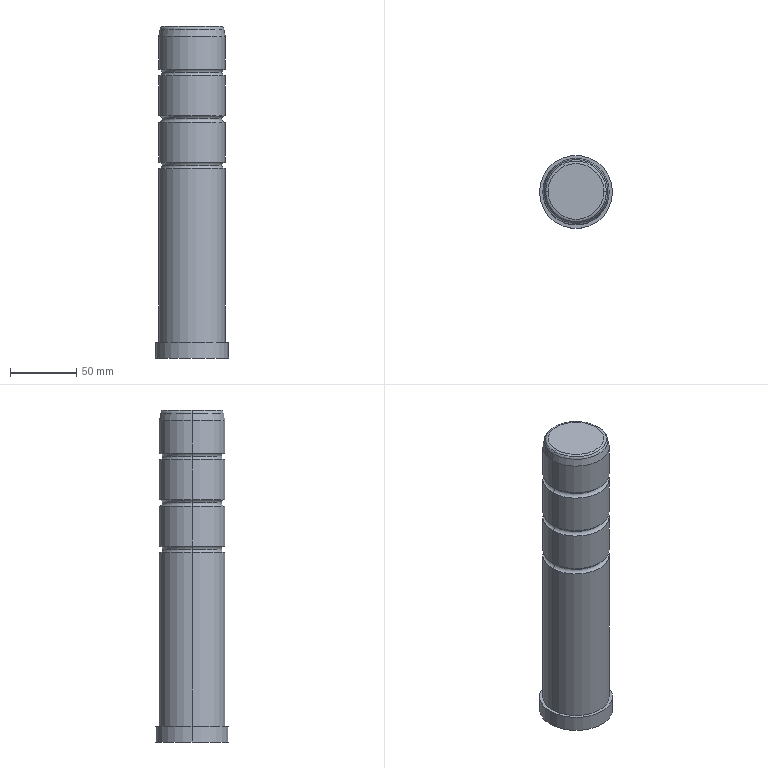Part | Creo | 1 solid | 31 faces | box 55 x 55 x 250 mm | volume 490289 mm3 | torus 16 | cylinder 10 | plane 3 | cone 2 | commonest cylinder face diameters 50 x8 55 x2
STEP:
#1=CARTESIAN_POINT('',(247.,347.,57.));
#2=VERTEX_POINT('',#1);
#3=CARTESIAN_POINT('',(297.,347.,57.));
#4=VERTEX_POINT('',#3);
#5=CARTESIAN_POINT('',(272.,347.,57.));
#6=DIRECTION('',(0.,0.,1.));
#7=DIRECTION('',(-1.,0.,0.));
#8=AXIS2_PLACEMENT_3D('',#5,#6,#7);
#9=CIRCLE('',#8,25.);
#10=EDGE_CURVE('',#2,#4,#9,.T.);
#11=ORIENTED_EDGE('',*,*,#10,.T.);
#12=CARTESIAN_POINT('',(297.,347.,27.));
#13=VERTEX_POINT('',#12);
#14=CARTESIAN_POINT('',(297.,347.,27.));
#15=DIRECTION('',(0.,0.,1.));
#16=VECTOR('',#15,30.);
#17=LINE('',#14,#16);
#18=EDGE_CURVE('',#13,#4,#17,.T.);
#19=ORIENTED_EDGE('',*,*,#18,.F.);
#20=CARTESIAN_POINT('',(247.,347.,27.));
#21=VERTEX_POINT('',#20);
#22=CARTESIAN_POINT('',(272.,347.,27.));
#23=DIRECTION('',(0.,0.,-1.));
#24=DIRECTION('',(1.,0.,0.));
#25=AXIS2_PLACEMENT_3D('',#22,#23,#24);
#26=CIRCLE('',#25,25.);
#27=EDGE_CURVE('',#13,#21,#26,.T.);
#28=ORIENTED_EDGE('',*,*,#27,.T.);
#29=CARTESIAN_POINT('',(247.,347.,27.));
#30=DIRECTION('',(0.,0.,1.));
#31=VECTOR('',#30,30.);
#32=LINE('',#29,#31);
#33=EDGE_CURVE('',#21,#2,#32,.T.);
#34=ORIENTED_EDGE('',*,*,#33,.T.);
#35=EDGE_LOOP('',(#11,#19,#28,#34));
#36=FACE_OUTER_BOUND('',#35,.F.);
#37=CARTESIAN_POINT('',(272.,347.,-108.5));
#38=DIRECTION('',(0.,0.,1.));
#39=DIRECTION('',(-1.,0.,0.));
#40=AXIS2_PLACEMENT_3D('',#37,#38,#39);
#41=CYLINDRICAL_SURFACE('',#40,25.);
#42=ADVANCED_FACE('',(#36),#41,.T.);
#43=ORIENTED_EDGE('',*,*,#10,.F.);
#44=CARTESIAN_POINT('',(249.5,347.,59.5));
#45=VERTEX_POINT('',#44);
#46=CARTESIAN_POINT('',(247.,347.,59.5));
#47=DIRECTION('',(0.,1.,0.));
#48=DIRECTION('',(1.,0.,0.));
#49=AXIS2_PLACEMENT_3D('',#46,#47,#48);
#50=CIRCLE('',#49,2.5);
#51=EDGE_CURVE('',#45,#2,#50,.T.);
#52=ORIENTED_EDGE('',*,*,#51,.F.);
#53=CARTESIAN_POINT('',(294.5,347.,59.5));
#54=VERTEX_POINT('',#53);
#55=CARTESIAN_POINT('',(272.,347.,59.5));
#56=DIRECTION('',(0.,0.,1.));
#57=DIRECTION('',(-1.,0.,0.));
#58=AXIS2_PLACEMENT_3D('',#55,#56,#57);
#59=CIRCLE('',#58,22.5);
#60=EDGE_CURVE('',#45,#54,#59,.T.);
#61=ORIENTED_EDGE('',*,*,#60,.T.);
#62=CARTESIAN_POINT('',(297.,347.,59.5));
#63=DIRECTION('',(0.,-1.,0.));
#64=DIRECTION('',(-1.,0.,0.));
#65=AXIS2_PLACEMENT_3D('',#62,#63,#64);
#66=CIRCLE('',#65,2.5);
#67=EDGE_CURVE('',#54,#4,#66,.T.);
#68=ORIENTED_EDGE('',*,*,#67,.T.);
#69=EDGE_LOOP('',(#43,#52,#61,#68));
#70=FACE_OUTER_BOUND('',#69,.F.);
#71=CARTESIAN_POINT('',(272.,347.,59.5));
#72=DIRECTION('',(0.,0.,1.));
#73=DIRECTION('',(-1.,0.,0.));
#74=AXIS2_PLACEMENT_3D('',#71,#72,#73);
#75=TOROIDAL_SURFACE('',#74,25.,2.5);
#76=ADVANCED_FACE('',(#70),#75,.F.);
#77=CARTESIAN_POINT('',(272.,347.,57.));
#78=DIRECTION('',(0.,0.,1.));
#79=DIRECTION('',(1.,0.,0.));
#80=AXIS2_PLACEMENT_3D('',#77,#78,#79);
#81=CIRCLE('',#80,25.);
#82=EDGE_CURVE('',#4,#2,#81,.T.);
#83=ORIENTED_EDGE('',*,*,#82,.F.);
#84=ORIENTED_EDGE('',*,*,#67,.F.);
#85=CARTESIAN_POINT('',(272.,347.,59.5));
#86=DIRECTION('',(0.,0.,1.));
#87=DIRECTION('',(1.,0.,0.));
#88=AXIS2_PLACEMENT_3D('',#85,#86,#87);
#89=CIRCLE('',#88,22.5);
#90=EDGE_CURVE('',#54,#45,#89,.T.);
#91=ORIENTED_EDGE('',*,*,#90,.T.);
#92=ORIENTED_EDGE('',*,*,#51,.T.);
#93=EDGE_LOOP('',(#83,#84,#91,#92));
#94=FACE_OUTER_BOUND('',#93,.F.);
#95=CARTESIAN_POINT('',(272.,347.,59.5));
#96=DIRECTION('',(0.,0.,1.));
#97=DIRECTION('',(-1.,0.,0.));
#98=AXIS2_PLACEMENT_3D('',#95,#96,#97);
#99=TOROIDAL_SURFACE('',#98,25.,2.5);
#100=ADVANCED_FACE('',(#94),#99,.F.);
#101=ORIENTED_EDGE('',*,*,#82,.T.);
#102=ORIENTED_EDGE('',*,*,#33,.F.);
#103=CARTESIAN_POINT('',(272.,347.,27.));
#104=DIRECTION('',(0.,0.,-1.));
#105=DIRECTION('',(-1.,0.,0.));
#106=AXIS2_PLACEMENT_3D('',#103,#104,#105);
#107=CIRCLE('',#106,25.);
#108=EDGE_CURVE('',#21,#13,#107,.T.);
#109=ORIENTED_EDGE('',*,*,#108,.T.);
#110=ORIENTED_EDGE('',*,*,#18,.T.);
#111=EDGE_LOOP('',(#101,#102,#109,#110));
#112=FACE_OUTER_BOUND('',#111,.F.);
#113=CARTESIAN_POINT('',(272.,347.,-108.5));
#114=DIRECTION('',(0.,0.,1.));
#115=DIRECTION('',(-1.,0.,0.));
#116=AXIS2_PLACEMENT_3D('',#113,#114,#115);
#117=CYLINDRICAL_SURFACE('',#116,25.);
#118=ADVANCED_FACE('',(#112),#117,.T.);
#119=ORIENTED_EDGE('',*,*,#108,.F.);
#120=CARTESIAN_POINT('',(249.5,347.,24.5));
#121=VERTEX_POINT('',#120);
#122=CARTESIAN_POINT('',(247.,347.,24.5));
#123=DIRECTION('',(0.,1.,0.));
#124=DIRECTION('',(0.,0.,1.));
#125=AXIS2_PLACEMENT_3D('',#122,#123,#124);
#126=CIRCLE('',#125,2.5);
#127=EDGE_CURVE('',#21,#121,#126,.T.);
#128=ORIENTED_EDGE('',*,*,#127,.T.);
#129=CARTESIAN_POINT('',(294.5,347.,24.5));
#130=VERTEX_POINT('',#129);
#131=CARTESIAN_POINT('',(272.,347.,24.5));
#132=DIRECTION('',(0.,0.,1.));
#133=DIRECTION('',(1.,0.,0.));
#134=AXIS2_PLACEMENT_3D('',#131,#132,#133);
#135=CIRCLE('',#134,22.5);
#136=EDGE_CURVE('',#130,#121,#135,.T.);
#137=ORIENTED_EDGE('',*,*,#136,.F.);
#138=CARTESIAN_POINT('',(297.,347.,24.5));
#139=DIRECTION('',(0.,-1.,0.));
#140=DIRECTION('',(0.,0.,1.));
#141=AXIS2_PLACEMENT_3D('',#138,#139,#140);
#142=CIRCLE('',#141,2.5);
#143=EDGE_CURVE('',#13,#130,#142,.T.);
#144=ORIENTED_EDGE('',*,*,#143,.F.);
#145=EDGE_LOOP('',(#119,#128,#137,#144));
#146=FACE_OUTER_BOUND('',#145,.F.);
#147=CARTESIAN_POINT('',(272.,347.,24.5));
#148=DIRECTION('',(0.,0.,1.));
#149=DIRECTION('',(-1.,0.,0.));
#150=AXIS2_PLACEMENT_3D('',#147,#148,#149);
#151=TOROIDAL_SURFACE('',#150,25.,2.5);
#152=ADVANCED_FACE('',(#146),#151,.F.);
#153=ORIENTED_EDGE('',*,*,#27,.F.);
#154=ORIENTED_EDGE('',*,*,#143,.T.);
#155=CARTESIAN_POINT('',(272.,347.,24.5));
#156=DIRECTION('',(0.,0.,1.));
#157=DIRECTION('',(-1.,0.,0.));
#158=AXIS2_PLACEMENT_3D('',#155,#156,#157);
#159=CIRCLE('',#158,22.5);
#160=EDGE_CURVE('',#121,#130,#159,.T.);
#161=ORIENTED_EDGE('',*,*,#160,.F.);
#162=ORIENTED_EDGE('',*,*,#127,.F.);
#163=EDGE_LOOP('',(#153,#154,#161,#162));
#164=FACE_OUTER_BOUND('',#163,.F.);
#165=CARTESIAN_POINT('',(272.,347.,24.5));
#166=DIRECTION('',(0.,0.,1.));
#167=DIRECTION('',(-1.,0.,0.));
#168=AXIS2_PLACEMENT_3D('',#165,#166,#167);
#169=TOROIDAL_SURFACE('',#168,25.,2.5);
#170=ADVANCED_FACE('',(#164),#169,.F.);
#171=CARTESIAN_POINT('',(247.,347.,22.));
#172=VERTEX_POINT('',#171);
#173=CARTESIAN_POINT('',(297.,347.,22.));
#174=VERTEX_POINT('',#173);
#175=CARTESIAN_POINT('',(272.,347.,22.));
#176=DIRECTION('',(0.,0.,1.));
#177=DIRECTION('',(-1.,0.,0.));
#178=AXIS2_PLACEMENT_3D('',#175,#176,#177);
#179=CIRCLE('',#178,25.);
#180=EDGE_CURVE('',#172,#174,#179,.T.);
#181=ORIENTED_EDGE('',*,*,#180,.F.);
#182=CARTESIAN_POINT('',(247.,347.,24.5));
#183=DIRECTION('',(0.,1.,0.));
#184=DIRECTION('',(1.,0.,0.));
#185=AXIS2_PLACEMENT_3D('',#182,#183,#184);
#186=CIRCLE('',#185,2.5);
#187=EDGE_CURVE('',#121,#172,#186,.T.);
#188=ORIENTED_EDGE('',*,*,#187,.F.);
#189=ORIENTED_EDGE('',*,*,#160,.T.);
#190=CARTESIAN_POINT('',(297.,347.,24.5));
#191=DIRECTION('',(0.,-1.,0.));
#192=DIRECTION('',(-1.,0.,0.));
#193=AXIS2_PLACEMENT_3D('',#190,#191,#192);
#194=CIRCLE('',#193,2.5);
#195=EDGE_CURVE('',#130,#174,#194,.T.);
#196=ORIENTED_EDGE('',*,*,#195,.T.);
#197=EDGE_LOOP('',(#181,#188,#189,#196));
#198=FACE_OUTER_BOUND('',#197,.F.);
#199=CARTESIAN_POINT('',(272.,347.,24.5));
#200=DIRECTION('',(0.,0.,1.));
#201=DIRECTION('',(-1.,0.,0.));
#202=AXIS2_PLACEMENT_3D('',#199,#200,#201);
#203=TOROIDAL_SURFACE('',#202,25.,2.5);
#204=ADVANCED_FACE('',(#198),#203,.F.);
#205=CARTESIAN_POINT('',(297.,347.,-108.5));
#206=VERTEX_POINT('',#205);
#207=CARTESIAN_POINT('',(247.,347.,-108.5));
#208=VERTEX_POINT('',#207);
#209=CARTESIAN_POINT('',(272.,347.,-108.5));
#210=DIRECTION('',(0.,0.,-1.));
#211=DIRECTION('',(1.,0.,0.));
#212=AXIS2_PLACEMENT_3D('',#209,#210,#211);
#213=CIRCLE('',#212,25.);
#214=EDGE_CURVE('',#206,#208,#213,.T.);
#215=ORIENTED_EDGE('',*,*,#214,.T.);
#216=CARTESIAN_POINT('',(247.,347.,-108.5));
#217=DIRECTION('',(0.,0.,1.));
#218=VECTOR('',#217,130.5);
#219=LINE('',#216,#218);
#220=EDGE_CURVE('',#208,#172,#219,.T.);
#221=ORIENTED_EDGE('',*,*,#220,.T.);
#222=ORIENTED_EDGE('',*,*,#180,.T.);
#223=CARTESIAN_POINT('',(297.,347.,-108.5));
#224=DIRECTION('',(0.,0.,1.));
#225=VECTOR('',#224,130.5);
#226=LINE('',#223,#225);
#227=EDGE_CURVE('',#206,#174,#226,.T.);
#228=ORIENTED_EDGE('',*,*,#227,.F.);
#229=EDGE_LOOP('',(#215,#221,#222,#228));
#230=FACE_OUTER_BOUND('',#229,.F.);
#231=CARTESIAN_POINT('',(272.,347.,-108.5));
#232=DIRECTION('',(0.,0.,1.));
#233=DIRECTION('',(-1.,0.,0.));
#234=AXIS2_PLACEMENT_3D('',#231,#232,#233);
#235=CYLINDRICAL_SURFACE('',#234,25.);
#236=ADVANCED_FACE('',(#230),#235,.T.);
#237=CARTESIAN_POINT('',(299.5,347.,-108.5));
#238=VERTEX_POINT('',#237);
#239=CARTESIAN_POINT('',(244.5,347.,-108.5));
#240=VERTEX_POINT('',#239);
#241=CARTESIAN_POINT('',(272.,347.,-108.5));
#242=DIRECTION('',(0.,0.,1.));
#243=DIRECTION('',(1.,0.,0.));
#244=AXIS2_PLACEMENT_3D('',#241,#242,#243);
#245=CIRCLE('',#244,27.5);
#246=EDGE_CURVE('',#238,#240,#245,.T.);
#247=ORIENTED_EDGE('',*,*,#246,.F.);
#248=CARTESIAN_POINT('',(272.,347.,-108.5));
#249=DIRECTION('',(0.,0.,1.));
#250=DIRECTION('',(-1.,0.,0.));
#251=AXIS2_PLACEMENT_3D('',#248,#249,#250);
#252=CIRCLE('',#251,27.5);
#253=EDGE_CURVE('',#240,#238,#252,.T.);
#254=ORIENTED_EDGE('',*,*,#253,.F.);
#255=EDGE_LOOP('',(#247,#254));
#256=FACE_OUTER_BOUND('',#255,.F.);
#257=CARTESIAN_POINT('',(272.,347.,-108.5));
#258=DIRECTION('',(0.,0.,-1.));
#259=DIRECTION('',(-1.,0.,0.));
#260=AXIS2_PLACEMENT_3D('',#257,#258,#259);
#261=CIRCLE('',#260,25.);
#262=EDGE_CURVE('',#208,#206,#261,.T.);
#263=ORIENTED_EDGE('',*,*,#262,.F.);
#264=ORIENTED_EDGE('',*,*,#214,.F.);
#265=EDGE_LOOP('',(#263,#264));
#266=FACE_BOUND('',#265,.F.);
#267=CARTESIAN_POINT('',(272.,347.,-108.5));
#268=DIRECTION('',(0.,0.,-1.));
#269=DIRECTION('',(1.,0.,0.));
#270=AXIS2_PLACEMENT_3D('',#267,#268,#269);
#271=PLANE('',#270);
#272=ADVANCED_FACE('',(#256,#266),#271,.F.);
#273=ORIENTED_EDGE('',*,*,#262,.T.);
#274=ORIENTED_EDGE('',*,*,#227,.T.);
#275=CARTESIAN_POINT('',(272.,347.,22.));
#276=DIRECTION('',(0.,0.,1.));
#277=DIRECTION('',(1.,0.,0.));
#278=AXIS2_PLACEMENT_3D('',#275,#276,#277);
#279=CIRCLE('',#278,25.);
#280=EDGE_CURVE('',#174,#172,#279,.T.);
#281=ORIENTED_EDGE('',*,*,#280,.T.);
#282=ORIENTED_EDGE('',*,*,#220,.F.);
#283=EDGE_LOOP('',(#273,#274,#281,#282));
#284=FACE_OUTER_BOUND('',#283,.F.);
#285=CARTESIAN_POINT('',(272.,347.,-108.5));
#286=DIRECTION('',(0.,0.,1.));
#287=DIRECTION('',(-1.,0.,0.));
#288=AXIS2_PLACEMENT_3D('',#285,#286,#287);
#289=CYLINDRICAL_SURFACE('',#288,25.);
#290=ADVANCED_FACE('',(#284),#289,.T.);
#291=ORIENTED_EDGE('',*,*,#280,.F.);
#292=ORIENTED_EDGE('',*,*,#195,.F.);
#293=ORIENTED_EDGE('',*,*,#136,.T.);
#294=ORIENTED_EDGE('',*,*,#187,.T.);
#295=EDGE_LOOP('',(#291,#292,#293,#294));
#296=FACE_OUTER_BOUND('',#295,.F.);
#297=CARTESIAN_POINT('',(272.,347.,24.5));
#298=DIRECTION('',(0.,0.,1.));
#299=DIRECTION('',(-1.,0.,0.));
#300=AXIS2_PLACEMENT_3D('',#297,#298,#299);
#301=TOROIDAL_SURFACE('',#300,25.,2.5);
#302=ADVANCED_FACE('',(#296),#301,.F.);
#303=ORIENTED_EDGE('',*,*,#246,.T.);
#304=CARTESIAN_POINT('',(244.5,347.,-120.5));
#305=VERTEX_POINT('',#304);
#306=CARTESIAN_POINT('',(244.5,347.,-108.5));
#307=DIRECTION('',(0.,0.,-1.));
#308=VECTOR('',#307,12.);
#309=LINE('',#306,#308);
#310=EDGE_CURVE('',#240,#305,#309,.T.);
#311=ORIENTED_EDGE('',*,*,#310,.T.);
#312=CARTESIAN_POINT('',(299.5,347.,-120.5));
#313=VERTEX_POINT('',#312);
#314=CARTESIAN_POINT('',(272.,347.,-120.5));
#315=DIRECTION('',(0.,0.,-1.));
#316=DIRECTION('',(-1.,0.,0.));
#317=AXIS2_PLACEMENT_3D('',#314,#315,#316);
#318=CIRCLE('',#317,27.5);
#319=EDGE_CURVE('',#305,#313,#318,.T.);
#320=ORIENTED_EDGE('',*,*,#319,.T.);
#321=CARTESIAN_POINT('',(299.5,347.,-108.5));
#322=DIRECTION('',(0.,0.,-1.));
#323=VECTOR('',#322,12.);
#324=LINE('',#321,#323);
#325=EDGE_CURVE('',#238,#313,#324,.T.);
#326=ORIENTED_EDGE('',*,*,#325,.F.);
#327=EDGE_LOOP('',(#303,#311,#320,#326));
#328=FACE_OUTER_BOUND('',#327,.F.);
#329=CARTESIAN_POINT('',(272.,347.,-108.5));
#330=DIRECTION('',(0.,0.,-1.));
#331=DIRECTION('',(1.,0.,0.));
#332=AXIS2_PLACEMENT_3D('',#329,#330,#331);
#333=CYLINDRICAL_SURFACE('',#332,27.5);
#334=ADVANCED_FACE('',(#328),#333,.T.);
#335=ORIENTED_EDGE('',*,*,#253,.T.);
#336=ORIENTED_EDGE('',*,*,#325,.T.);
#337=CARTESIAN_POINT('',(272.,347.,-120.5));
#338=DIRECTION('',(0.,0.,-1.));
#339=DIRECTION('',(1.,0.,0.));
#340=AXIS2_PLACEMENT_3D('',#337,#338,#339);
#341=CIRCLE('',#340,27.5);
#342=EDGE_CURVE('',#313,#305,#341,.T.);
#343=ORIENTED_EDGE('',*,*,#342,.T.);
#344=ORIENTED_EDGE('',*,*,#310,.F.);
#345=EDGE_LOOP('',(#335,#336,#343,#344));
#346=FACE_OUTER_BOUND('',#345,.F.);
#347=CARTESIAN_POINT('',(272.,347.,-108.5));
#348=DIRECTION('',(0.,0.,-1.));
#349=DIRECTION('',(1.,0.,0.));
#350=AXIS2_PLACEMENT_3D('',#347,#348,#349);
#351=CYLINDRICAL_SURFACE('',#350,27.5);
#352=ADVANCED_FACE('',(#346),#351,.T.);
#353=ORIENTED_EDGE('',*,*,#342,.F.);
#354=ORIENTED_EDGE('',*,*,#319,.F.);
#355=EDGE_LOOP('',(#353,#354));
#356=FACE_OUTER_BOUND('',#355,.F.);
#357=CARTESIAN_POINT('',(272.,347.,-120.5));
#358=DIRECTION('',(0.,0.,-1.));
#359=DIRECTION('',(1.,0.,0.));
#360=AXIS2_PLACEMENT_3D('',#357,#358,#359);
#361=PLANE('',#360);
#362=ADVANCED_FACE('',(#356),#361,.T.);
#363=CARTESIAN_POINT('',(247.,347.,62.));
#364=VERTEX_POINT('',#363);
#365=CARTESIAN_POINT('',(297.,347.,62.));
#366=VERTEX_POINT('',#365);
#367=CARTESIAN_POINT('',(272.,347.,62.));
#368=DIRECTION('',(0.,0.,-1.));
#369=DIRECTION('',(-1.,0.,0.));
#370=AXIS2_PLACEMENT_3D('',#367,#368,#369);
#371=CIRCLE('',#370,25.);
#372=EDGE_CURVE('',#364,#366,#371,.T.);
#373=ORIENTED_EDGE('',*,*,#372,.F.);
#374=CARTESIAN_POINT('',(247.,347.,59.5));
#375=DIRECTION('',(0.,1.,0.));
#376=DIRECTION('',(0.,0.,1.));
#377=AXIS2_PLACEMENT_3D('',#374,#375,#376);
#378=CIRCLE('',#377,2.5);
#379=EDGE_CURVE('',#364,#45,#378,.T.);
#380=ORIENTED_EDGE('',*,*,#379,.T.);
#381=ORIENTED_EDGE('',*,*,#90,.F.);
#382=CARTESIAN_POINT('',(297.,347.,59.5));
#383=DIRECTION('',(0.,-1.,0.));
#384=DIRECTION('',(0.,0.,1.));
#385=AXIS2_PLACEMENT_3D('',#382,#383,#384);
#386=CIRCLE('',#385,2.5);
#387=EDGE_CURVE('',#366,#54,#386,.T.);
#388=ORIENTED_EDGE('',*,*,#387,.F.);
#389=EDGE_LOOP('',(#373,#380,#381,#388));
#390=FACE_OUTER_BOUND('',#389,.F.);
#391=CARTESIAN_POINT('',(272.,347.,59.5));
#392=DIRECTION('',(0.,0.,1.));
#393=DIRECTION('',(-1.,0.,0.));
#394=AXIS2_PLACEMENT_3D('',#391,#392,#393);
#395=TOROIDAL_SURFACE('',#394,25.,2.5);
#396=ADVANCED_FACE('',(#390),#395,.F.);
#397=CARTESIAN_POINT('',(297.,347.,92.));
#398=VERTEX_POINT('',#397);
#399=CARTESIAN_POINT('',(247.,347.,92.));
#400=VERTEX_POINT('',#399);
#401=CARTESIAN_POINT('',(272.,347.,92.));
#402=DIRECTION('',(0.,0.,1.));
#403=DIRECTION('',(1.,0.,0.));
#404=AXIS2_PLACEMENT_3D('',#401,#402,#403);
#405=CIRCLE('',#404,25.);
#406=EDGE_CURVE('',#398,#400,#405,.T.);
#407=ORIENTED_EDGE('',*,*,#406,.T.);
#408=CARTESIAN_POINT('',(247.,347.,62.));
#409=DIRECTION('',(0.,0.,1.));
#410=VECTOR('',#409,30.);
#411=LINE('',#408,#410);
#412=EDGE_CURVE('',#364,#400,#411,.T.);
#413=ORIENTED_EDGE('',*,*,#412,.F.);
#414=ORIENTED_EDGE('',*,*,#372,.T.);
#415=CARTESIAN_POINT('',(297.,347.,62.));
#416=DIRECTION('',(0.,0.,1.));
#417=VECTOR('',#416,30.);
#418=LINE('',#415,#417);
#419=EDGE_CURVE('',#366,#398,#418,.T.);
#420=ORIENTED_EDGE('',*,*,#419,.T.);
#421=EDGE_LOOP('',(#407,#413,#414,#420));
#422=FACE_OUTER_BOUND('',#421,.F.);
#423=CARTESIAN_POINT('',(272.,347.,-108.5));
#424=DIRECTION('',(0.,0.,1.));
#425=DIRECTION('',(-1.,0.,0.));
#426=AXIS2_PLACEMENT_3D('',#423,#424,#425);
#427=CYLINDRICAL_SURFACE('',#426,25.);
#428=ADVANCED_FACE('',(#422),#427,.T.);
#429=ORIENTED_EDGE('',*,*,#406,.F.);
#430=CARTESIAN_POINT('',(294.5,347.,94.5));
#431=VERTEX_POINT('',#430);
#432=CARTESIAN_POINT('',(297.,347.,94.5));
#433=DIRECTION('',(0.,-1.,0.));
#434=DIRECTION('',(-1.,0.,0.));
#435=AXIS2_PLACEMENT_3D('',#432,#433,#434);
#436=CIRCLE('',#435,2.5);
#437=EDGE_CURVE('',#431,#398,#436,.T.);
#438=ORIENTED_EDGE('',*,*,#437,.F.);
#439=CARTESIAN_POINT('',(249.5,347.,94.5));
#440=VERTEX_POINT('',#439);
#441=CARTESIAN_POINT('',(272.,347.,94.5));
#442=DIRECTION('',(0.,0.,1.));
#443=DIRECTION('',(1.,0.,0.));
#444=AXIS2_PLACEMENT_3D('',#441,#442,#443);
#445=CIRCLE('',#444,22.5);
#446=EDGE_CURVE('',#431,#440,#445,.T.);
#447=ORIENTED_EDGE('',*,*,#446,.T.);
#448=CARTESIAN_POINT('',(247.,347.,94.5));
#449=DIRECTION('',(0.,1.,0.));
#450=DIRECTION('',(1.,0.,0.));
#451=AXIS2_PLACEMENT_3D('',#448,#449,#450);
#452=CIRCLE('',#451,2.5);
#453=EDGE_CURVE('',#440,#400,#452,.T.);
#454=ORIENTED_EDGE('',*,*,#453,.T.);
#455=EDGE_LOOP('',(#429,#438,#447,#454));
#456=FACE_OUTER_BOUND('',#455,.F.);
#457=CARTESIAN_POINT('',(272.,347.,94.5));
#458=DIRECTION('',(0.,0.,1.));
#459=DIRECTION('',(-1.,0.,0.));
#460=AXIS2_PLACEMENT_3D('',#457,#458,#459);
#461=TOROIDAL_SURFACE('',#460,25.,2.5);
#462=ADVANCED_FACE('',(#456),#461,.F.);
#463=CARTESIAN_POINT('',(272.,347.,92.));
#464=DIRECTION('',(0.,0.,1.));
#465=DIRECTION('',(-1.,0.,0.));
#466=AXIS2_PLACEMENT_3D('',#463,#464,#465);
#467=CIRCLE('',#466,25.);
#468=EDGE_CURVE('',#400,#398,#467,.T.);
#469=ORIENTED_EDGE('',*,*,#468,.F.);
#470=ORIENTED_EDGE('',*,*,#453,.F.);
#471=CARTESIAN_POINT('',(272.,347.,94.5));
#472=DIRECTION('',(0.,0.,1.));
#473=DIRECTION('',(-1.,0.,0.));
#474=AXIS2_PLACEMENT_3D('',#471,#472,#473);
#475=CIRCLE('',#474,22.5);
#476=EDGE_CURVE('',#440,#431,#475,.T.);
#477=ORIENTED_EDGE('',*,*,#476,.T.);
#478=ORIENTED_EDGE('',*,*,#437,.T.);
#479=EDGE_LOOP('',(#469,#470,#477,#478));
#480=FACE_OUTER_BOUND('',#479,.F.);
#481=CARTESIAN_POINT('',(272.,347.,94.5));
#482=DIRECTION('',(0.,0.,1.));
#483=DIRECTION('',(-1.,0.,0.));
#484=AXIS2_PLACEMENT_3D('',#481,#482,#483);
#485=TOROIDAL_SURFACE('',#484,25.,2.5);
#486=ADVANCED_FACE('',(#480),#485,.F.);
#487=ORIENTED_EDGE('',*,*,#468,.T.);
#488=ORIENTED_EDGE('',*,*,#419,.F.);
#489=CARTESIAN_POINT('',(272.,347.,62.));
#490=DIRECTION('',(0.,0.,-1.));
#491=DIRECTION('',(1.,0.,0.));
#492=AXIS2_PLACEMENT_3D('',#489,#490,#491);
#493=CIRCLE('',#492,25.);
#494=EDGE_CURVE('',#366,#364,#493,.T.);
#495=ORIENTED_EDGE('',*,*,#494,.T.);
#496=ORIENTED_EDGE('',*,*,#412,.T.);
#497=EDGE_LOOP('',(#487,#488,#495,#496));
#498=FACE_OUTER_BOUND('',#497,.F.);
#499=CARTESIAN_POINT('',(272.,347.,-108.5));
#500=DIRECTION('',(0.,0.,1.));
#501=DIRECTION('',(-1.,0.,0.));
#502=AXIS2_PLACEMENT_3D('',#499,#500,#501);
#503=CYLINDRICAL_SURFACE('',#502,25.);
#504=ADVANCED_FACE('',(#498),#503,.T.);
#505=ORIENTED_EDGE('',*,*,#494,.F.);
#506=ORIENTED_EDGE('',*,*,#387,.T.);
#507=ORIENTED_EDGE('',*,*,#60,.F.);
#508=ORIENTED_EDGE('',*,*,#379,.F.);
#509=EDGE_LOOP('',(#505,#506,#507,#508));
#510=FACE_OUTER_BOUND('',#509,.F.);
#511=CARTESIAN_POINT('',(272.,347.,59.5));
#512=DIRECTION('',(0.,0.,1.));
#513=DIRECTION('',(-1.,0.,0.));
#514=AXIS2_PLACEMENT_3D('',#511,#512,#513);
#515=TOROIDAL_SURFACE('',#514,25.,2.5);
#516=ADVANCED_FACE('',(#510),#515,.F.);
#517=CARTESIAN_POINT('',(297.,347.,97.));
#518=VERTEX_POINT('',#517);
#519=CARTESIAN_POINT('',(247.,347.,97.));
#520=VERTEX_POINT('',#519);
#521=CARTESIAN_POINT('',(272.,347.,97.));
#522=DIRECTION('',(0.,0.,-1.));
#523=DIRECTION('',(1.,0.,0.));
#524=AXIS2_PLACEMENT_3D('',#521,#522,#523);
#525=CIRCLE('',#524,25.);
#526=EDGE_CURVE('',#518,#520,#525,.T.);
#527=ORIENTED_EDGE('',*,*,#526,.F.);
#528=CARTESIAN_POINT('',(297.,347.,94.5));
#529=DIRECTION('',(0.,-1.,0.));
#530=DIRECTION('',(0.,0.,1.));
#531=AXIS2_PLACEMENT_3D('',#528,#529,#530);
#532=CIRCLE('',#531,2.5);
#533=EDGE_CURVE('',#518,#431,#532,.T.);
#534=ORIENTED_EDGE('',*,*,#533,.T.);
#535=ORIENTED_EDGE('',*,*,#476,.F.);
#536=CARTESIAN_POINT('',(247.,347.,94.5));
#537=DIRECTION('',(0.,1.,0.));
#538=DIRECTION('',(0.,0.,1.));
#539=AXIS2_PLACEMENT_3D('',#536,#537,#538);
#540=CIRCLE('',#539,2.5);
#541=EDGE_CURVE('',#520,#440,#540,.T.);
#542=ORIENTED_EDGE('',*,*,#541,.F.);
#543=EDGE_LOOP('',(#527,#534,#535,#542));
#544=FACE_OUTER_BOUND('',#543,.F.);
#545=CARTESIAN_POINT('',(272.,347.,94.5));
#546=DIRECTION('',(0.,0.,1.));
#547=DIRECTION('',(-1.,0.,0.));
#548=AXIS2_PLACEMENT_3D('',#545,#546,#547);
#549=TOROIDAL_SURFACE('',#548,25.,2.5);
#550=ADVANCED_FACE('',(#544),#549,.F.);
#551=ORIENTED_EDGE('',*,*,#526,.T.);
#552=CARTESIAN_POINT('',(247.,347.,121.5));
#553=VERTEX_POINT('',#552);
#554=CARTESIAN_POINT('',(247.,347.,97.));
#555=DIRECTION('',(0.,0.,1.));
#556=VECTOR('',#555,24.5);
#557=LINE('',#554,#556);
#558=EDGE_CURVE('',#520,#553,#557,.T.);
#559=ORIENTED_EDGE('',*,*,#558,.T.);
#560=CARTESIAN_POINT('',(297.,347.,121.5));
#561=VERTEX_POINT('',#560);
#562=CARTESIAN_POINT('',(272.,347.,121.5));
#563=DIRECTION('',(0.,0.,1.));
#564=DIRECTION('',(-1.,0.,0.));
#565=AXIS2_PLACEMENT_3D('',#562,#563,#564);
#566=CIRCLE('',#565,25.);
#567=EDGE_CURVE('',#553,#561,#566,.T.);
#568=ORIENTED_EDGE('',*,*,#567,.T.);
#569=CARTESIAN_POINT('',(297.,347.,97.));
#570=DIRECTION('',(0.,0.,1.));
#571=VECTOR('',#570,24.5);
#572=LINE('',#569,#571);
#573=EDGE_CURVE('',#518,#561,#572,.T.);
#574=ORIENTED_EDGE('',*,*,#573,.F.);
#575=EDGE_LOOP('',(#551,#559,#568,#574));
#576=FACE_OUTER_BOUND('',#575,.F.);
#577=CARTESIAN_POINT('',(272.,347.,-108.5));
#578=DIRECTION('',(0.,0.,1.));
#579=DIRECTION('',(-1.,0.,0.));
#580=AXIS2_PLACEMENT_3D('',#577,#578,#579);
#581=CYLINDRICAL_SURFACE('',#580,25.);
#582=ADVANCED_FACE('',(#576),#581,.T.);
#583=CARTESIAN_POINT('',(272.,347.,97.));
#584=DIRECTION('',(0.,0.,-1.));
#585=DIRECTION('',(-1.,0.,0.));
#586=AXIS2_PLACEMENT_3D('',#583,#584,#585);
#587=CIRCLE('',#586,25.);
#588=EDGE_CURVE('',#520,#518,#587,.T.);
#589=ORIENTED_EDGE('',*,*,#588,.T.);
#590=ORIENTED_EDGE('',*,*,#573,.T.);
#591=CARTESIAN_POINT('',(272.,347.,121.5));
#592=DIRECTION('',(0.,0.,1.));
#593=DIRECTION('',(1.,0.,0.));
#594=AXIS2_PLACEMENT_3D('',#591,#592,#593);
#595=CIRCLE('',#594,25.);
#596=EDGE_CURVE('',#561,#553,#595,.T.);
#597=ORIENTED_EDGE('',*,*,#596,.T.);
#598=ORIENTED_EDGE('',*,*,#558,.F.);
#599=EDGE_LOOP('',(#589,#590,#597,#598));
#600=FACE_OUTER_BOUND('',#599,.F.);
#601=CARTESIAN_POINT('',(272.,347.,-108.5));
#602=DIRECTION('',(0.,0.,1.));
#603=DIRECTION('',(-1.,0.,0.));
#604=AXIS2_PLACEMENT_3D('',#601,#602,#603);
#605=CYLINDRICAL_SURFACE('',#604,25.);
#606=ADVANCED_FACE('',(#600),#605,.T.);
#607=ORIENTED_EDGE('',*,*,#588,.F.);
#608=ORIENTED_EDGE('',*,*,#541,.T.);
#609=ORIENTED_EDGE('',*,*,#446,.F.);
#610=ORIENTED_EDGE('',*,*,#533,.F.);
#611=EDGE_LOOP('',(#607,#608,#609,#610));
#612=FACE_OUTER_BOUND('',#611,.F.);
#613=CARTESIAN_POINT('',(272.,347.,94.5));
#614=DIRECTION('',(0.,0.,1.));
#615=DIRECTION('',(-1.,0.,0.));
#616=AXIS2_PLACEMENT_3D('',#613,#614,#615);
#617=TOROIDAL_SURFACE('',#616,25.,2.5);
#618=ADVANCED_FACE('',(#612),#617,.F.);
#619=CARTESIAN_POINT('',(295.959,347.,127.053));
#620=VERTEX_POINT('',#619);
#621=CARTESIAN_POINT('',(248.041,347.,127.053));
#622=VERTEX_POINT('',#621);
#623=CARTESIAN_POINT('',(272.,347.,127.053));
#624=DIRECTION('',(0.,0.,1.));
#625=DIRECTION('',(1.,0.,0.));
#626=AXIS2_PLACEMENT_3D('',#623,#624,#625);
#627=CIRCLE('',#626,23.959);
#628=EDGE_CURVE('',#620,#622,#627,.T.);
#629=ORIENTED_EDGE('',*,*,#628,.T.);
#630=CARTESIAN_POINT('',(248.041,347.,127.053));
#631=DIRECTION('',(-0.1843,0.,-0.9829));
#632=VECTOR('',#631,5.65);
#633=LINE('',#630,#632);
#634=EDGE_CURVE('',#622,#553,#633,.T.);
#635=ORIENTED_EDGE('',*,*,#634,.T.);
#636=ORIENTED_EDGE('',*,*,#596,.F.);
#637=CARTESIAN_POINT('',(295.959,347.,127.053));
#638=DIRECTION('',(0.1843,0.,-0.9829));
#639=VECTOR('',#638,5.65);
#640=LINE('',#637,#639);
#641=EDGE_CURVE('',#620,#561,#640,.T.);
#642=ORIENTED_EDGE('',*,*,#641,.F.);
#643=EDGE_LOOP('',(#629,#635,#636,#642));
#644=FACE_OUTER_BOUND('',#643,.F.);
#645=CARTESIAN_POINT('',(272.,347.,124.276));
#646=DIRECTION('',(0.,0.,-1.));
#647=DIRECTION('',(1.,0.,0.));
#648=AXIS2_PLACEMENT_3D('',#645,#646,#647);
#649=CONICAL_SURFACE('',#648,24.479,10.62);
#650=ADVANCED_FACE('',(#644),#649,.T.);
#651=ORIENTED_EDGE('',*,*,#628,.F.);
#652=CARTESIAN_POINT('',(294.926,347.,128.809));
#653=VERTEX_POINT('',#652);
#654=CARTESIAN_POINT('',(293.01,347.,126.5));
#655=DIRECTION('',(0.,-1.,0.));
#656=DIRECTION('',(0.9829,0.,0.1843));
#657=AXIS2_PLACEMENT_3D('',#654,#655,#656);
#658=CIRCLE('',#657,3.);
#659=EDGE_CURVE('',#620,#653,#658,.T.);
#660=ORIENTED_EDGE('',*,*,#659,.T.);
#661=CARTESIAN_POINT('',(249.074,347.,128.809));
#662=VERTEX_POINT('',#661);
#663=CARTESIAN_POINT('',(272.,347.,128.809));
#664=DIRECTION('',(0.,0.,1.));
#665=DIRECTION('',(1.,0.,0.));
#666=AXIS2_PLACEMENT_3D('',#663,#664,#665);
#667=CIRCLE('',#666,22.926);
#668=EDGE_CURVE('',#653,#662,#667,.T.);
#669=ORIENTED_EDGE('',*,*,#668,.T.);
#670=CARTESIAN_POINT('',(250.99,347.,126.5));
#671=DIRECTION('',(0.,1.,0.));
#672=DIRECTION('',(-0.9829,0.,0.1843));
#673=AXIS2_PLACEMENT_3D('',#670,#671,#672);
#674=CIRCLE('',#673,3.);
#675=EDGE_CURVE('',#622,#662,#674,.T.);
#676=ORIENTED_EDGE('',*,*,#675,.F.);
#677=EDGE_LOOP('',(#651,#660,#669,#676));
#678=FACE_OUTER_BOUND('',#677,.F.);
#679=CARTESIAN_POINT('',(272.,347.,126.5));
#680=DIRECTION('',(0.,0.,1.));
#681=DIRECTION('',(-1.,0.,0.));
#682=AXIS2_PLACEMENT_3D('',#679,#680,#681);
#683=TOROIDAL_SURFACE('',#682,21.01,3.);
#684=ADVANCED_FACE('',(#678),#683,.T.);
#685=CARTESIAN_POINT('',(272.,347.,127.053));
#686=DIRECTION('',(0.,0.,1.));
#687=DIRECTION('',(-1.,0.,0.));
#688=AXIS2_PLACEMENT_3D('',#685,#686,#687);
#689=CIRCLE('',#688,23.959);
#690=EDGE_CURVE('',#622,#620,#689,.T.);
#691=ORIENTED_EDGE('',*,*,#690,.F.);
#692=ORIENTED_EDGE('',*,*,#675,.T.);
#693=CARTESIAN_POINT('',(272.,347.,128.809));
#694=DIRECTION('',(0.,0.,1.));
#695=DIRECTION('',(-1.,0.,0.));
#696=AXIS2_PLACEMENT_3D('',#693,#694,#695);
#697=CIRCLE('',#696,22.926);
#698=EDGE_CURVE('',#662,#653,#697,.T.);
#699=ORIENTED_EDGE('',*,*,#698,.T.);
#700=ORIENTED_EDGE('',*,*,#659,.F.);
#701=EDGE_LOOP('',(#691,#692,#699,#700));
#702=FACE_OUTER_BOUND('',#701,.F.);
#703=CARTESIAN_POINT('',(272.,347.,126.5));
#704=DIRECTION('',(0.,0.,1.));
#705=DIRECTION('',(-1.,0.,0.));
#706=AXIS2_PLACEMENT_3D('',#703,#704,#705);
#707=TOROIDAL_SURFACE('',#706,21.01,3.);
#708=ADVANCED_FACE('',(#702),#707,.T.);
#709=ORIENTED_EDGE('',*,*,#690,.T.);
#710=ORIENTED_EDGE('',*,*,#641,.T.);
#711=ORIENTED_EDGE('',*,*,#567,.F.);
#712=ORIENTED_EDGE('',*,*,#634,.F.);
#713=EDGE_LOOP('',(#709,#710,#711,#712));
#714=FACE_OUTER_BOUND('',#713,.F.);
#715=CARTESIAN_POINT('',(272.,347.,124.276));
#716=DIRECTION('',(0.,0.,-1.));
#717=DIRECTION('',(1.,0.,0.));
#718=AXIS2_PLACEMENT_3D('',#715,#716,#717);
#719=CONICAL_SURFACE('',#718,24.479,10.62);
#720=ADVANCED_FACE('',(#714),#719,.T.);
#721=CARTESIAN_POINT('',(250.99,347.,129.5));
#722=VERTEX_POINT('',#721);
#723=CARTESIAN_POINT('',(293.01,347.,129.5));
#724=VERTEX_POINT('',#723);
#725=CARTESIAN_POINT('',(272.,347.,129.5));
#726=DIRECTION('',(0.,0.,1.));
#727=DIRECTION('',(-1.,0.,0.));
#728=AXIS2_PLACEMENT_3D('',#725,#726,#727);
#729=CIRCLE('',#728,21.01);
#730=EDGE_CURVE('',#722,#724,#729,.T.);
#731=ORIENTED_EDGE('',*,*,#730,.T.);
#732=CARTESIAN_POINT('',(293.01,347.,126.5));
#733=DIRECTION('',(0.,-1.,0.));
#734=DIRECTION('',(0.6386,0.,0.7695));
#735=AXIS2_PLACEMENT_3D('',#732,#733,#734);
#736=CIRCLE('',#735,3.);
#737=EDGE_CURVE('',#653,#724,#736,.T.);
#738=ORIENTED_EDGE('',*,*,#737,.F.);
#739=ORIENTED_EDGE('',*,*,#698,.F.);
#740=CARTESIAN_POINT('',(250.99,347.,126.5));
#741=DIRECTION('',(0.,1.,0.));
#742=DIRECTION('',(-0.6386,0.,0.7695));
#743=AXIS2_PLACEMENT_3D('',#740,#741,#742);
#744=CIRCLE('',#743,3.);
#745=EDGE_CURVE('',#662,#722,#744,.T.);
#746=ORIENTED_EDGE('',*,*,#745,.T.);
#747=EDGE_LOOP('',(#731,#738,#739,#746));
#748=FACE_OUTER_BOUND('',#747,.F.);
#749=CARTESIAN_POINT('',(272.,347.,126.5));
#750=DIRECTION('',(0.,0.,1.));
#751=DIRECTION('',(-1.,0.,0.));
#752=AXIS2_PLACEMENT_3D('',#749,#750,#751);
#753=TOROIDAL_SURFACE('',#752,21.01,3.);
#754=ADVANCED_FACE('',(#748),#753,.T.);
#755=ORIENTED_EDGE('',*,*,#730,.F.);
#756=CARTESIAN_POINT('',(272.,347.,129.5));
#757=DIRECTION('',(0.,0.,1.));
#758=DIRECTION('',(1.,0.,0.));
#759=AXIS2_PLACEMENT_3D('',#756,#757,#758);
#760=CIRCLE('',#759,21.01);
#761=EDGE_CURVE('',#724,#722,#760,.T.);
#762=ORIENTED_EDGE('',*,*,#761,.F.);
#763=EDGE_LOOP('',(#755,#762));
#764=FACE_OUTER_BOUND('',#763,.F.);
#765=CARTESIAN_POINT('',(272.,347.,129.5));
#766=DIRECTION('',(0.,0.,1.));
#767=DIRECTION('',(-1.,0.,0.));
#768=AXIS2_PLACEMENT_3D('',#765,#766,#767);
#769=PLANE('',#768);
#770=ADVANCED_FACE('',(#764),#769,.T.);
#771=ORIENTED_EDGE('',*,*,#761,.T.);
#772=ORIENTED_EDGE('',*,*,#745,.F.);
#773=ORIENTED_EDGE('',*,*,#668,.F.);
#774=ORIENTED_EDGE('',*,*,#737,.T.);
#775=EDGE_LOOP('',(#771,#772,#773,#774));
#776=FACE_OUTER_BOUND('',#775,.F.);
#777=CARTESIAN_POINT('',(272.,347.,126.5));
#778=DIRECTION('',(0.,0.,1.));
#779=DIRECTION('',(-1.,0.,0.));
#780=AXIS2_PLACEMENT_3D('',#777,#778,#779);
#781=TOROIDAL_SURFACE('',#780,21.01,3.);
#782=ADVANCED_FACE('',(#776),#781,.T.);
#783=CLOSED_SHELL('',(#42,#76,#100,#118,#152,#170,#204,#236,#272,#290,#302,#334,#352,#362,#396,#428,#462,#486,#504,#516,#550,#582,#606,#618,#650,#684,#708,#720,#754,#770,#782));
#784=MANIFOLD_SOLID_BREP('',#783);
#785=(LENGTH_UNIT()NAMED_UNIT(*)SI_UNIT(.MILLI.,.METRE.));
#786=UNCERTAINTY_MEASURE_WITH_UNIT(LENGTH_MEASURE(0.02618),#785,'','');
#787=(NAMED_UNIT(*)PLANE_ANGLE_UNIT()SI_UNIT($,.RADIAN.));
#788=PLANE_ANGLE_MEASURE_WITH_UNIT(PLANE_ANGLE_MEASURE(0.01745),#787);
#789=(CONVERSION_BASED_UNIT('DEGREE',#788)NAMED_UNIT(*)PLANE_ANGLE_UNIT());
#790=(NAMED_UNIT(*)SI_UNIT($,.STERADIAN.)SOLID_ANGLE_UNIT());
#791=(GEOMETRIC_REPRESENTATION_CONTEXT(3)GLOBAL_UNCERTAINTY_ASSIGNED_CONTEXT((#786))GLOBAL_UNIT_ASSIGNED_CONTEXT((#785,#789,#790))REPRESENTATION_CONTEXT('',''));
#792=ADVANCED_BREP_SHAPE_REPRESENTATION('',(#784),#791);